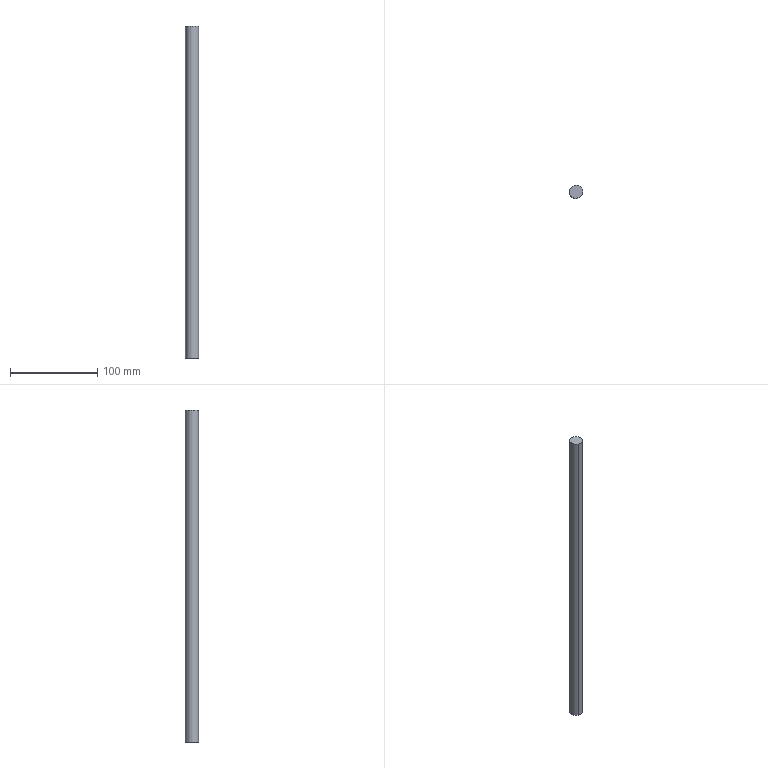Part | STEP file | Boss-Extrude 1-3 | 1 solid | 4 faces | box 15 x 15 x 380 mm | volume 67152 mm3 | cylinder 2 | plane 2 | commonest cylinder face diameters 15 x2
STEP:
#1=CARTESIAN_POINT('',(-1395.567,1821.061,2896.751));
#2=VERTEX_POINT('',#1);
#3=CARTESIAN_POINT('',(-1401.909,1807.468,2896.751));
#4=VERTEX_POINT('',#3);
#5=CARTESIAN_POINT('',(-1398.738,1814.264,2896.751));
#6=DIRECTION('',(0.,0.,1.));
#7=DIRECTION('',(0.4228,0.9062,0.));
#8=AXIS2_PLACEMENT_3D('',#5,#6,#7);
#9=CIRCLE('',#8,7.5);
#10=EDGE_CURVE('',#2,#4,#9,.T.);
#11=ORIENTED_EDGE('',*,*,#10,.F.);
#12=CARTESIAN_POINT('',(-1395.567,1821.061,2516.751));
#13=VERTEX_POINT('',#12);
#14=CARTESIAN_POINT('',(-1395.567,1821.061,2896.751));
#15=DIRECTION('',(0.,0.,-1.));
#16=VECTOR('',#15,1000.);
#17=LINE('',#14,#16);
#18=EDGE_CURVE('',#2,#13,#17,.T.);
#19=ORIENTED_EDGE('',*,*,#18,.T.);
#20=CARTESIAN_POINT('',(-1401.909,1807.468,2516.751));
#21=VERTEX_POINT('',#20);
#22=CARTESIAN_POINT('',(-1398.738,1814.264,2516.751));
#23=DIRECTION('',(0.,0.,1.));
#24=DIRECTION('',(0.4228,0.9062,0.));
#25=AXIS2_PLACEMENT_3D('',#22,#23,#24);
#26=CIRCLE('',#25,7.5);
#27=EDGE_CURVE('',#13,#21,#26,.T.);
#28=ORIENTED_EDGE('',*,*,#27,.T.);
#29=CARTESIAN_POINT('',(-1401.909,1807.468,2896.751));
#30=DIRECTION('',(0.,0.,-1.));
#31=VECTOR('',#30,1000.);
#32=LINE('',#29,#31);
#33=EDGE_CURVE('',#4,#21,#32,.T.);
#34=ORIENTED_EDGE('',*,*,#33,.F.);
#35=EDGE_LOOP('',(#11,#19,#28,#34));
#36=FACE_OUTER_BOUND('',#35,.T.);
#37=CARTESIAN_POINT('',(-1398.738,1814.264,2896.751));
#38=DIRECTION('',(0.,0.,-1.));
#39=DIRECTION('',(0.4228,0.9062,0.));
#40=AXIS2_PLACEMENT_3D('',#37,#38,#39);
#41=CYLINDRICAL_SURFACE('',#40,7.5);
#42=ADVANCED_FACE('',(#36),#41,.T.);
#43=ORIENTED_EDGE('',*,*,#18,.F.);
#44=CARTESIAN_POINT('',(-1398.738,1814.264,2896.751));
#45=DIRECTION('',(0.,0.,1.));
#46=DIRECTION('',(0.4228,0.9062,0.));
#47=AXIS2_PLACEMENT_3D('',#44,#45,#46);
#48=CIRCLE('',#47,7.5);
#49=EDGE_CURVE('',#4,#2,#48,.T.);
#50=ORIENTED_EDGE('',*,*,#49,.F.);
#51=ORIENTED_EDGE('',*,*,#33,.T.);
#52=CARTESIAN_POINT('',(-1398.738,1814.264,2516.751));
#53=DIRECTION('',(0.,0.,1.));
#54=DIRECTION('',(0.4228,0.9062,0.));
#55=AXIS2_PLACEMENT_3D('',#52,#53,#54);
#56=CIRCLE('',#55,7.5);
#57=EDGE_CURVE('',#21,#13,#56,.T.);
#58=ORIENTED_EDGE('',*,*,#57,.T.);
#59=EDGE_LOOP('',(#43,#50,#51,#58));
#60=FACE_OUTER_BOUND('',#59,.T.);
#61=CARTESIAN_POINT('',(-1398.738,1814.264,2896.751));
#62=DIRECTION('',(0.,0.,-1.));
#63=DIRECTION('',(0.4228,0.9062,0.));
#64=AXIS2_PLACEMENT_3D('',#61,#62,#63);
#65=CYLINDRICAL_SURFACE('',#64,7.5);
#66=ADVANCED_FACE('',(#60),#65,.T.);
#67=ORIENTED_EDGE('',*,*,#49,.T.);
#68=ORIENTED_EDGE('',*,*,#10,.T.);
#69=EDGE_LOOP('',(#67,#68));
#70=FACE_OUTER_BOUND('',#69,.T.);
#71=CARTESIAN_POINT('',(-1398.738,1814.264,2896.751));
#72=DIRECTION('',(0.,0.,1.));
#73=DIRECTION('',(-0.4228,-0.9062,0.));
#74=AXIS2_PLACEMENT_3D('',#71,#72,#73);
#75=PLANE('',#74);
#76=ADVANCED_FACE('',(#70),#75,.T.);
#77=ORIENTED_EDGE('',*,*,#57,.F.);
#78=ORIENTED_EDGE('',*,*,#27,.F.);
#79=EDGE_LOOP('',(#77,#78));
#80=FACE_OUTER_BOUND('',#79,.T.);
#81=CARTESIAN_POINT('',(-1398.738,1814.264,2516.751));
#82=DIRECTION('',(0.,0.,1.));
#83=DIRECTION('',(-0.4228,-0.9062,0.));
#84=AXIS2_PLACEMENT_3D('',#81,#82,#83);
#85=PLANE('',#84);
#86=ADVANCED_FACE('',(#80),#85,.F.);
#87=CLOSED_SHELL('',(#42,#66,#76,#86));
#88=MANIFOLD_SOLID_BREP('',#87);
#89=CARTESIAN_POINT('',(0.,0.,0.));
#90=DIRECTION('',(0.,0.,1.));
#91=DIRECTION('',(1.,0.,0.));
#92=AXIS2_PLACEMENT_3D('',#89,#90,#91);
#93=(LENGTH_UNIT()NAMED_UNIT(*)SI_UNIT(.MILLI.,.METRE.));
#94=UNCERTAINTY_MEASURE_WITH_UNIT(LENGTH_MEASURE(0.00001),#93,'','');
#95=(NAMED_UNIT(*)PLANE_ANGLE_UNIT()SI_UNIT($,.RADIAN.));
#96=(NAMED_UNIT(*)SI_UNIT($,.STERADIAN.)SOLID_ANGLE_UNIT());
#97=(GEOMETRIC_REPRESENTATION_CONTEXT(3)GLOBAL_UNCERTAINTY_ASSIGNED_CONTEXT((#94))GLOBAL_UNIT_ASSIGNED_CONTEXT((#93,#95,#96))REPRESENTATION_CONTEXT('',''));
#98=ADVANCED_BREP_SHAPE_REPRESENTATION('',(#88,#92),#97);